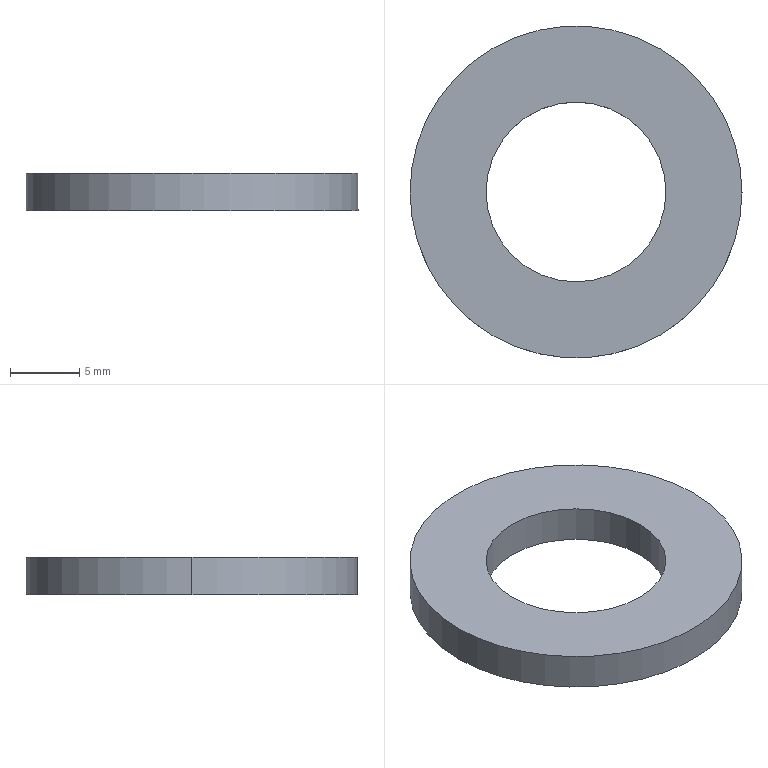Part | STEP file | Pin washer nut at M12 | 1 solid | 6 faces | box 24 x 24 x 2.7 mm | volume 863.074 mm3 | cylinder 4 | plane 2 | commonest cylinder face diameters 13 x2 24 x2
STEP:
#1=CARTESIAN_POINT('',(-6.5,0.,2.7));
#2=VERTEX_POINT('',#1);
#3=CARTESIAN_POINT('',(6.5,0.,2.7));
#4=VERTEX_POINT('',#3);
#5=CARTESIAN_POINT('',(0.,0.,2.7));
#6=DIRECTION('',(0.,0.,1.));
#7=DIRECTION('',(1.,0.,0.));
#8=AXIS2_PLACEMENT_3D('',#5,#6,#7);
#9=CIRCLE('',#8,6.5);
#10=EDGE_CURVE('',#2,#4,#9,.T.);
#11=ORIENTED_EDGE('',*,*,#10,.T.);
#12=CARTESIAN_POINT('',(6.5,0.,0.));
#13=VERTEX_POINT('',#12);
#14=CARTESIAN_POINT('',(6.5,0.,2.7));
#15=DIRECTION('',(0.,0.,-1.));
#16=VECTOR('',#15,1000.);
#17=LINE('',#14,#16);
#18=EDGE_CURVE('',#4,#13,#17,.T.);
#19=ORIENTED_EDGE('',*,*,#18,.T.);
#20=CARTESIAN_POINT('',(-6.5,0.,0.));
#21=VERTEX_POINT('',#20);
#22=CARTESIAN_POINT('',(0.,0.,0.));
#23=DIRECTION('',(0.,0.,1.));
#24=DIRECTION('',(1.,0.,0.));
#25=AXIS2_PLACEMENT_3D('',#22,#23,#24);
#26=CIRCLE('',#25,6.5);
#27=EDGE_CURVE('',#21,#13,#26,.T.);
#28=ORIENTED_EDGE('',*,*,#27,.F.);
#29=CARTESIAN_POINT('',(-6.5,0.,2.7));
#30=DIRECTION('',(0.,0.,-1.));
#31=VECTOR('',#30,1000.);
#32=LINE('',#29,#31);
#33=EDGE_CURVE('',#2,#21,#32,.T.);
#34=ORIENTED_EDGE('',*,*,#33,.F.);
#35=EDGE_LOOP('',(#11,#19,#28,#34));
#36=FACE_OUTER_BOUND('',#35,.T.);
#37=CARTESIAN_POINT('',(0.,0.,2.7));
#38=DIRECTION('',(0.,0.,-1.));
#39=DIRECTION('',(-1.,0.,0.));
#40=AXIS2_PLACEMENT_3D('',#37,#38,#39);
#41=CYLINDRICAL_SURFACE('',#40,6.5);
#42=ADVANCED_FACE('',(#36),#41,.F.);
#43=CARTESIAN_POINT('',(12.,0.,2.7));
#44=VERTEX_POINT('',#43);
#45=CARTESIAN_POINT('',(-12.,0.,2.7));
#46=VERTEX_POINT('',#45);
#47=CARTESIAN_POINT('',(0.,0.,2.7));
#48=DIRECTION('',(0.,0.,1.));
#49=DIRECTION('',(1.,0.,0.));
#50=AXIS2_PLACEMENT_3D('',#47,#48,#49);
#51=CIRCLE('',#50,12.);
#52=EDGE_CURVE('',#44,#46,#51,.T.);
#53=ORIENTED_EDGE('',*,*,#52,.F.);
#54=CARTESIAN_POINT('',(12.,0.,0.));
#55=VERTEX_POINT('',#54);
#56=CARTESIAN_POINT('',(12.,0.,2.7));
#57=DIRECTION('',(0.,0.,-1.));
#58=VECTOR('',#57,1000.);
#59=LINE('',#56,#58);
#60=EDGE_CURVE('',#44,#55,#59,.T.);
#61=ORIENTED_EDGE('',*,*,#60,.T.);
#62=CARTESIAN_POINT('',(-12.,0.,0.));
#63=VERTEX_POINT('',#62);
#64=CARTESIAN_POINT('',(0.,0.,0.));
#65=DIRECTION('',(0.,0.,1.));
#66=DIRECTION('',(1.,0.,0.));
#67=AXIS2_PLACEMENT_3D('',#64,#65,#66);
#68=CIRCLE('',#67,12.);
#69=EDGE_CURVE('',#55,#63,#68,.T.);
#70=ORIENTED_EDGE('',*,*,#69,.T.);
#71=CARTESIAN_POINT('',(-12.,0.,2.7));
#72=DIRECTION('',(0.,0.,-1.));
#73=VECTOR('',#72,1000.);
#74=LINE('',#71,#73);
#75=EDGE_CURVE('',#46,#63,#74,.T.);
#76=ORIENTED_EDGE('',*,*,#75,.F.);
#77=EDGE_LOOP('',(#53,#61,#70,#76));
#78=FACE_OUTER_BOUND('',#77,.T.);
#79=CARTESIAN_POINT('',(0.,0.,2.7));
#80=DIRECTION('',(0.,0.,-1.));
#81=DIRECTION('',(-1.,0.,0.));
#82=AXIS2_PLACEMENT_3D('',#79,#80,#81);
#83=CYLINDRICAL_SURFACE('',#82,12.);
#84=ADVANCED_FACE('',(#78),#83,.T.);
#85=CARTESIAN_POINT('',(0.,0.,2.7));
#86=DIRECTION('',(0.,0.,1.));
#87=DIRECTION('',(1.,0.,0.));
#88=AXIS2_PLACEMENT_3D('',#85,#86,#87);
#89=CIRCLE('',#88,12.);
#90=EDGE_CURVE('',#46,#44,#89,.T.);
#91=ORIENTED_EDGE('',*,*,#90,.T.);
#92=ORIENTED_EDGE('',*,*,#52,.T.);
#93=EDGE_LOOP('',(#91,#92));
#94=FACE_OUTER_BOUND('',#93,.T.);
#95=ORIENTED_EDGE('',*,*,#10,.F.);
#96=CARTESIAN_POINT('',(0.,0.,2.7));
#97=DIRECTION('',(0.,0.,1.));
#98=DIRECTION('',(1.,0.,0.));
#99=AXIS2_PLACEMENT_3D('',#96,#97,#98);
#100=CIRCLE('',#99,6.5);
#101=EDGE_CURVE('',#4,#2,#100,.T.);
#102=ORIENTED_EDGE('',*,*,#101,.F.);
#103=EDGE_LOOP('',(#95,#102));
#104=FACE_BOUND('',#103,.T.);
#105=CARTESIAN_POINT('',(0.,0.,2.7));
#106=DIRECTION('',(0.,0.,1.));
#107=DIRECTION('',(1.,0.,0.));
#108=AXIS2_PLACEMENT_3D('',#105,#106,#107);
#109=PLANE('',#108);
#110=ADVANCED_FACE('',(#94,#104),#109,.T.);
#111=CARTESIAN_POINT('',(0.,0.,0.));
#112=DIRECTION('',(0.,0.,1.));
#113=DIRECTION('',(1.,0.,0.));
#114=AXIS2_PLACEMENT_3D('',#111,#112,#113);
#115=CIRCLE('',#114,12.);
#116=EDGE_CURVE('',#63,#55,#115,.T.);
#117=ORIENTED_EDGE('',*,*,#116,.F.);
#118=ORIENTED_EDGE('',*,*,#69,.F.);
#119=EDGE_LOOP('',(#117,#118));
#120=FACE_OUTER_BOUND('',#119,.T.);
#121=ORIENTED_EDGE('',*,*,#27,.T.);
#122=CARTESIAN_POINT('',(0.,0.,0.));
#123=DIRECTION('',(0.,0.,1.));
#124=DIRECTION('',(1.,0.,0.));
#125=AXIS2_PLACEMENT_3D('',#122,#123,#124);
#126=CIRCLE('',#125,6.5);
#127=EDGE_CURVE('',#13,#21,#126,.T.);
#128=ORIENTED_EDGE('',*,*,#127,.T.);
#129=EDGE_LOOP('',(#121,#128));
#130=FACE_BOUND('',#129,.T.);
#131=CARTESIAN_POINT('',(0.,0.,0.));
#132=DIRECTION('',(0.,0.,1.));
#133=DIRECTION('',(1.,0.,0.));
#134=AXIS2_PLACEMENT_3D('',#131,#132,#133);
#135=PLANE('',#134);
#136=ADVANCED_FACE('',(#120,#130),#135,.F.);
#137=ORIENTED_EDGE('',*,*,#60,.F.);
#138=ORIENTED_EDGE('',*,*,#90,.F.);
#139=ORIENTED_EDGE('',*,*,#75,.T.);
#140=ORIENTED_EDGE('',*,*,#116,.T.);
#141=EDGE_LOOP('',(#137,#138,#139,#140));
#142=FACE_OUTER_BOUND('',#141,.T.);
#143=CARTESIAN_POINT('',(0.,0.,2.7));
#144=DIRECTION('',(0.,0.,-1.));
#145=DIRECTION('',(-1.,0.,0.));
#146=AXIS2_PLACEMENT_3D('',#143,#144,#145);
#147=CYLINDRICAL_SURFACE('',#146,12.);
#148=ADVANCED_FACE('',(#142),#147,.T.);
#149=ORIENTED_EDGE('',*,*,#18,.F.);
#150=ORIENTED_EDGE('',*,*,#101,.T.);
#151=ORIENTED_EDGE('',*,*,#33,.T.);
#152=ORIENTED_EDGE('',*,*,#127,.F.);
#153=EDGE_LOOP('',(#149,#150,#151,#152));
#154=FACE_OUTER_BOUND('',#153,.T.);
#155=CARTESIAN_POINT('',(0.,0.,2.7));
#156=DIRECTION('',(0.,0.,-1.));
#157=DIRECTION('',(-1.,0.,0.));
#158=AXIS2_PLACEMENT_3D('',#155,#156,#157);
#159=CYLINDRICAL_SURFACE('',#158,6.5);
#160=ADVANCED_FACE('',(#154),#159,.F.);
#161=CLOSED_SHELL('',(#42,#84,#110,#136,#148,#160));
#162=MANIFOLD_SOLID_BREP('',#161);
#163=CARTESIAN_POINT('',(0.,0.,0.));
#164=DIRECTION('',(0.,0.,1.));
#165=DIRECTION('',(1.,0.,0.));
#166=AXIS2_PLACEMENT_3D('',#163,#164,#165);
#167=(LENGTH_UNIT()NAMED_UNIT(*)SI_UNIT(.MILLI.,.METRE.));
#168=UNCERTAINTY_MEASURE_WITH_UNIT(LENGTH_MEASURE(0.00001),#167,'','');
#169=(NAMED_UNIT(*)PLANE_ANGLE_UNIT()SI_UNIT($,.RADIAN.));
#170=(NAMED_UNIT(*)SI_UNIT($,.STERADIAN.)SOLID_ANGLE_UNIT());
#171=(GEOMETRIC_REPRESENTATION_CONTEXT(3)GLOBAL_UNCERTAINTY_ASSIGNED_CONTEXT((#168))GLOBAL_UNIT_ASSIGNED_CONTEXT((#167,#169,#170))REPRESENTATION_CONTEXT('',''));
#172=ADVANCED_BREP_SHAPE_REPRESENTATION('',(#162,#166),#171);